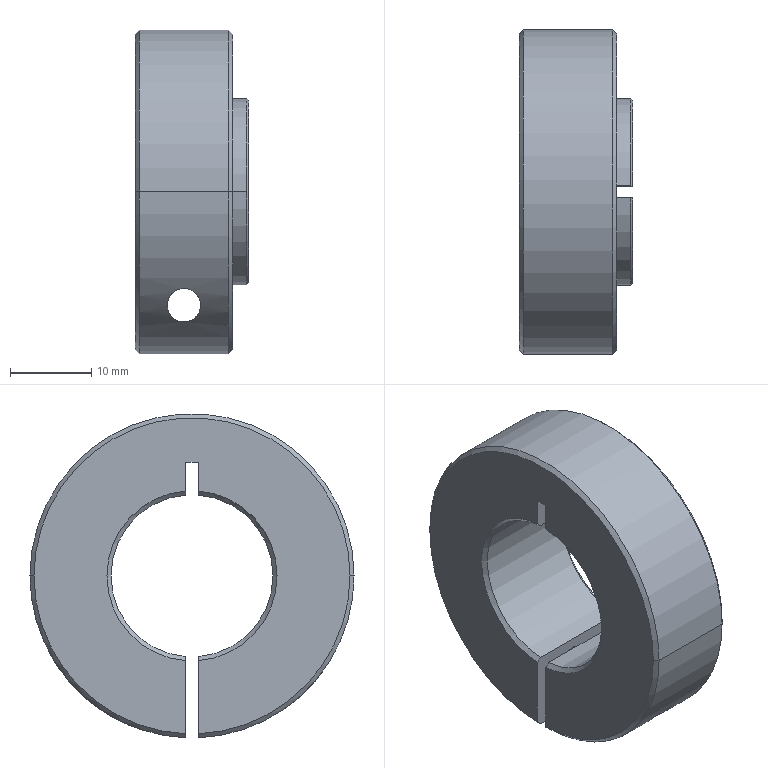Part | NX | features 1_11 2 | 1 solid | 42 faces | box 14 x 40 x 39.986 mm | volume 10434 mm3 | cone 17 | cylinder 15 | plane 10 | commonest cylinder face diameters 20 x3 23 x3 40 x3 4.134 x2 5.5 x2 9 x2
STEP:
#1=CARTESIAN_POINT('',(-38.25,-260.05,-709.529));
#2=VERTEX_POINT('',#1);
#3=CARTESIAN_POINT('',(-32.75,-260.05,-709.529));
#4=VERTEX_POINT('',#3);
#5=CARTESIAN_POINT('',(-35.5,-260.05,-709.529));
#6=DIRECTION('',(0.,1.,0.));
#7=DIRECTION('',(-1.,0.,0.));
#8=AXIS2_PLACEMENT_3D('',#5,#6,#7);
#9=CIRCLE('',#8,2.75);
#10=EDGE_CURVE('',#2,#4,#9,.T.);
#11=ORIENTED_EDGE('',*,*,#10,.F.);
#12=CARTESIAN_POINT('',(-38.25,-253.8,-709.529));
#13=VERTEX_POINT('',#12);
#14=CARTESIAN_POINT('',(-38.25,-253.8,-709.529));
#15=DIRECTION('',(0.,-1.,0.));
#16=VECTOR('',#15,1000.);
#17=LINE('',#14,#16);
#18=EDGE_CURVE('',#13,#2,#17,.T.);
#19=ORIENTED_EDGE('',*,*,#18,.F.);
#20=CARTESIAN_POINT('',(-32.75,-253.8,-709.529));
#21=VERTEX_POINT('',#20);
#22=CARTESIAN_POINT('',(-35.5,-253.8,-709.529));
#23=DIRECTION('',(0.,-1.,0.));
#24=DIRECTION('',(1.,0.,0.));
#25=AXIS2_PLACEMENT_3D('',#22,#23,#24);
#26=CIRCLE('',#25,2.75);
#27=EDGE_CURVE('',#21,#13,#26,.T.);
#28=ORIENTED_EDGE('',*,*,#27,.F.);
#29=CARTESIAN_POINT('',(-32.75,-253.8,-709.529));
#30=DIRECTION('',(0.,-1.,0.));
#31=VECTOR('',#30,1000.);
#32=LINE('',#29,#31);
#33=EDGE_CURVE('',#4,#21,#32,.F.);
#34=ORIENTED_EDGE('',*,*,#33,.F.);
#35=EDGE_LOOP('',(#11,#19,#28,#34));
#36=FACE_BOUND('',#35,.T.);
#37=CARTESIAN_POINT('',(-35.5,-257.3,-709.529));
#38=DIRECTION('',(0.,1.,0.));
#39=DIRECTION('',(-1.,0.,0.));
#40=AXIS2_PLACEMENT_3D('',#37,#38,#39);
#41=CYLINDRICAL_SURFACE('',#40,2.75);
#42=ADVANCED_FACE('',(#36),#41,.F.);
#43=CARTESIAN_POINT('',(-27.5,-261.55,-684.279));
#44=VERTEX_POINT('',#43);
#45=CARTESIAN_POINT('',(-27.5,-272.075,-695.529));
#46=VERTEX_POINT('',#45);
#47=CARTESIAN_POINT('',(-27.5,-260.8,-695.529));
#48=DIRECTION('',(1.,0.,0.));
#49=DIRECTION('',(0.,-0.06652,0.9978));
#50=AXIS2_PLACEMENT_3D('',#47,#48,#49);
#51=CIRCLE('',#50,11.275);
#52=EDGE_CURVE('',#44,#46,#51,.T.);
#53=ORIENTED_EDGE('',*,*,#52,.F.);
#54=CARTESIAN_POINT('',(-27.725,-261.55,-684.054));
#55=VERTEX_POINT('',#54);
#56=CARTESIAN_POINT('',(-27.725,-261.55,-684.054));
#57=CARTESIAN_POINT('',(-27.65,-261.55,-684.129));
#58=CARTESIAN_POINT('',(-27.575,-261.55,-684.204));
#59=CARTESIAN_POINT('',(-27.5,-261.55,-684.279));
#60=B_SPLINE_CURVE_WITH_KNOTS('',3,(#56,#57,#58,#59),.UNSPECIFIED.,.F.,.F.,(4,4),(0.,1.),.UNSPECIFIED.);
#61=EDGE_CURVE('',#44,#55,#60,.F.);
#62=ORIENTED_EDGE('',*,*,#61,.T.);
#63=CARTESIAN_POINT('',(-27.725,-272.3,-695.529));
#64=VERTEX_POINT('',#63);
#65=CARTESIAN_POINT('',(-27.725,-260.8,-695.529));
#66=DIRECTION('',(1.,0.,0.));
#67=DIRECTION('',(0.,-0.06522,0.9979));
#68=AXIS2_PLACEMENT_3D('',#65,#66,#67);
#69=CIRCLE('',#68,11.5);
#70=EDGE_CURVE('',#55,#64,#69,.T.);
#71=ORIENTED_EDGE('',*,*,#70,.T.);
#72=CARTESIAN_POINT('',(-27.725,-272.3,-695.529));
#73=DIRECTION('',(0.7071,0.7071,0.));
#74=VECTOR('',#73,1000.);
#75=LINE('',#72,#74);
#76=EDGE_CURVE('',#64,#46,#75,.T.);
#77=ORIENTED_EDGE('',*,*,#76,.T.);
#78=EDGE_LOOP('',(#53,#62,#71,#77));
#79=FACE_BOUND('',#78,.T.);
#80=CARTESIAN_POINT('',(-27.451,-260.8,-695.529));
#81=DIRECTION('',(-1.,0.,0.));
#82=DIRECTION('',(0.,-1.,0.));
#83=AXIS2_PLACEMENT_3D('',#80,#81,#82);
#84=CONICAL_SURFACE('',#83,11.226,0.7854);
#85=ADVANCED_FACE('',(#79),#84,.T.);
#86=CARTESIAN_POINT('',(-29.5,-260.05,-715.015));
#87=VERTEX_POINT('',#86);
#88=CARTESIAN_POINT('',(-29.5,-241.3,-695.529));
#89=VERTEX_POINT('',#88);
#90=CARTESIAN_POINT('',(-29.5,-260.8,-695.529));
#91=DIRECTION('',(1.,0.,0.));
#92=DIRECTION('',(0.,0.03846,-0.9993));
#93=AXIS2_PLACEMENT_3D('',#90,#91,#92);
#94=CIRCLE('',#93,19.5);
#95=EDGE_CURVE('',#87,#89,#94,.T.);
#96=ORIENTED_EDGE('',*,*,#95,.F.);
#97=CARTESIAN_POINT('',(-30.,-260.05,-715.515));
#98=VERTEX_POINT('',#97);
#99=CARTESIAN_POINT('',(-30.,-260.05,-715.515));
#100=CARTESIAN_POINT('',(-29.833,-260.05,-715.349));
#101=CARTESIAN_POINT('',(-29.667,-260.05,-715.182));
#102=CARTESIAN_POINT('',(-29.5,-260.05,-715.015));
#103=B_SPLINE_CURVE_WITH_KNOTS('',3,(#99,#100,#101,#102),.UNSPECIFIED.,.F.,.F.,(4,4),(0.,1.),.UNSPECIFIED.);
#104=EDGE_CURVE('',#87,#98,#103,.F.);
#105=ORIENTED_EDGE('',*,*,#104,.T.);
#106=CARTESIAN_POINT('',(-30.,-240.8,-695.529));
#107=VERTEX_POINT('',#106);
#108=CARTESIAN_POINT('',(-30.,-260.8,-695.529));
#109=DIRECTION('',(1.,0.,0.));
#110=DIRECTION('',(0.,0.0375,-0.9993));
#111=AXIS2_PLACEMENT_3D('',#108,#109,#110);
#112=CIRCLE('',#111,20.);
#113=EDGE_CURVE('',#98,#107,#112,.T.);
#114=ORIENTED_EDGE('',*,*,#113,.T.);
#115=CARTESIAN_POINT('',(-30.,-240.8,-695.529));
#116=DIRECTION('',(0.7071,-0.7071,0.));
#117=VECTOR('',#116,1000.);
#118=LINE('',#115,#117);
#119=EDGE_CURVE('',#107,#89,#118,.T.);
#120=ORIENTED_EDGE('',*,*,#119,.T.);
#121=EDGE_LOOP('',(#96,#105,#114,#120));
#122=FACE_BOUND('',#121,.T.);
#123=CARTESIAN_POINT('',(-29.451,-260.8,-695.529));
#124=DIRECTION('',(-1.,0.,0.));
#125=DIRECTION('',(0.,-1.,0.));
#126=AXIS2_PLACEMENT_3D('',#123,#124,#125);
#127=CONICAL_SURFACE('',#126,19.451,0.7854);
#128=ADVANCED_FACE('',(#122),#127,.T.);
#129=CARTESIAN_POINT('',(-33.433,-261.983,-709.529));
#130=VERTEX_POINT('',#129);
#131=CARTESIAN_POINT('',(-37.567,-261.983,-709.529));
#132=VERTEX_POINT('',#131);
#133=CARTESIAN_POINT('',(-35.5,-261.983,-709.529));
#134=DIRECTION('',(0.,-1.,0.));
#135=DIRECTION('',(1.,0.,0.));
#136=AXIS2_PLACEMENT_3D('',#133,#134,#135);
#137=CIRCLE('',#136,2.067);
#138=EDGE_CURVE('',#130,#132,#137,.T.);
#139=ORIENTED_EDGE('',*,*,#138,.F.);
#140=CARTESIAN_POINT('',(-33.433,-275.083,-709.529));
#141=VERTEX_POINT('',#140);
#142=CARTESIAN_POINT('',(-33.433,-275.083,-709.529));
#143=DIRECTION('',(0.,1.,0.));
#144=VECTOR('',#143,1000.);
#145=LINE('',#142,#144);
#146=EDGE_CURVE('',#141,#130,#145,.T.);
#147=ORIENTED_EDGE('',*,*,#146,.F.);
#148=CARTESIAN_POINT('',(-37.567,-275.083,-709.529));
#149=VERTEX_POINT('',#148);
#150=CARTESIAN_POINT('',(-37.567,-275.083,-709.529));
#151=CARTESIAN_POINT('',(-37.567,-275.524,-709.078));
#152=CARTESIAN_POINT('',(-37.348,-276.166,-708.351));
#153=CARTESIAN_POINT('',(-36.445,-276.738,-707.615));
#154=CARTESIAN_POINT('',(-35.5,-276.906,-707.386));
#155=CARTESIAN_POINT('',(-34.555,-276.738,-707.615));
#156=CARTESIAN_POINT('',(-33.652,-276.166,-708.351));
#157=CARTESIAN_POINT('',(-33.433,-275.524,-709.078));
#158=CARTESIAN_POINT('',(-33.433,-275.083,-709.529));
#159=B_SPLINE_CURVE_WITH_KNOTS('',3,(#150,#151,#152,#153,#154,#155,#156,#157,#158),.UNSPECIFIED.,.F.,.F.,(4,1,1,1,1,1,4),(0.,0.25,0.375,0.5,0.625,0.75,1.),.UNSPECIFIED.);
#160=EDGE_CURVE('',#141,#149,#159,.F.);
#161=ORIENTED_EDGE('',*,*,#160,.T.);
#162=CARTESIAN_POINT('',(-37.567,-275.083,-709.529));
#163=DIRECTION('',(0.,1.,0.));
#164=VECTOR('',#163,1000.);
#165=LINE('',#162,#164);
#166=EDGE_CURVE('',#132,#149,#165,.F.);
#167=ORIENTED_EDGE('',*,*,#166,.F.);
#168=EDGE_LOOP('',(#139,#147,#161,#167));
#169=FACE_BOUND('',#168,.T.);
#170=CARTESIAN_POINT('',(-35.5,-272.267,-709.529));
#171=DIRECTION('',(0.,-1.,0.));
#172=DIRECTION('',(1.,0.,0.));
#173=AXIS2_PLACEMENT_3D('',#170,#171,#172);
#174=CYLINDRICAL_SURFACE('',#173,2.067);
#175=ADVANCED_FACE('',(#169),#174,.F.);
#176=ORIENTED_EDGE('',*,*,#138,.T.);
#177=CARTESIAN_POINT('',(-38.,-261.55,-709.529));
#178=VERTEX_POINT('',#177);
#179=CARTESIAN_POINT('',(-38.,-261.55,-709.529));
#180=DIRECTION('',(0.7071,-0.7071,0.));
#181=VECTOR('',#180,1000.);
#182=LINE('',#179,#181);
#183=EDGE_CURVE('',#178,#132,#182,.T.);
#184=ORIENTED_EDGE('',*,*,#183,.F.);
#185=CARTESIAN_POINT('',(-33.,-261.55,-709.529));
#186=VERTEX_POINT('',#185);
#187=CARTESIAN_POINT('',(-35.5,-261.55,-709.529));
#188=DIRECTION('',(0.,-1.,0.));
#189=DIRECTION('',(1.,0.,0.));
#190=AXIS2_PLACEMENT_3D('',#187,#188,#189);
#191=CIRCLE('',#190,2.5);
#192=EDGE_CURVE('',#186,#178,#191,.T.);
#193=ORIENTED_EDGE('',*,*,#192,.F.);
#194=CARTESIAN_POINT('',(-33.,-261.55,-709.529));
#195=DIRECTION('',(-0.7071,-0.7071,0.));
#196=VECTOR('',#195,1000.);
#197=LINE('',#194,#196);
#198=EDGE_CURVE('',#130,#186,#197,.F.);
#199=ORIENTED_EDGE('',*,*,#198,.F.);
#200=EDGE_LOOP('',(#176,#184,#193,#199));
#201=FACE_BOUND('',#200,.T.);
#202=CARTESIAN_POINT('',(-35.5,-262.032,-709.529));
#203=DIRECTION('',(0.,1.,0.));
#204=DIRECTION('',(-1.,0.,0.));
#205=AXIS2_PLACEMENT_3D('',#202,#203,#204);
#206=CONICAL_SURFACE('',#205,2.018,0.7854);
#207=ADVANCED_FACE('',(#201),#206,.F.);
#208=ORIENTED_EDGE('',*,*,#198,.T.);
#209=CARTESIAN_POINT('',(-35.5,-261.55,-709.529));
#210=DIRECTION('',(0.,-1.,0.));
#211=DIRECTION('',(-1.,0.,0.));
#212=AXIS2_PLACEMENT_3D('',#209,#210,#211);
#213=CIRCLE('',#212,2.5);
#214=EDGE_CURVE('',#178,#186,#213,.T.);
#215=ORIENTED_EDGE('',*,*,#214,.F.);
#216=ORIENTED_EDGE('',*,*,#183,.T.);
#217=CARTESIAN_POINT('',(-35.5,-261.983,-709.529));
#218=DIRECTION('',(0.,-1.,0.));
#219=DIRECTION('',(-1.,0.,0.));
#220=AXIS2_PLACEMENT_3D('',#217,#218,#219);
#221=CIRCLE('',#220,2.067);
#222=EDGE_CURVE('',#132,#130,#221,.T.);
#223=ORIENTED_EDGE('',*,*,#222,.T.);
#224=EDGE_LOOP('',(#208,#215,#216,#223));
#225=FACE_BOUND('',#224,.T.);
#226=CARTESIAN_POINT('',(-35.5,-262.032,-709.529));
#227=DIRECTION('',(0.,1.,0.));
#228=DIRECTION('',(-1.,0.,0.));
#229=AXIS2_PLACEMENT_3D('',#226,#227,#228);
#230=CONICAL_SURFACE('',#229,2.018,0.7854);
#231=ADVANCED_FACE('',(#225),#230,.F.);
#232=ORIENTED_EDGE('',*,*,#166,.T.);
#233=CARTESIAN_POINT('',(-33.433,-275.083,-709.529));
#234=CARTESIAN_POINT('',(-33.433,-274.603,-710.02));
#235=CARTESIAN_POINT('',(-33.683,-273.842,-710.714));
#236=CARTESIAN_POINT('',(-34.497,-272.96,-711.413));
#237=CARTESIAN_POINT('',(-35.5,-272.586,-711.688));
#238=CARTESIAN_POINT('',(-36.503,-272.96,-711.413));
#239=CARTESIAN_POINT('',(-37.317,-273.842,-710.714));
#240=CARTESIAN_POINT('',(-37.567,-274.603,-710.02));
#241=CARTESIAN_POINT('',(-37.567,-275.083,-709.529));
#242=B_SPLINE_CURVE_WITH_KNOTS('',3,(#233,#234,#235,#236,#237,#238,#239,#240,#241),.UNSPECIFIED.,.F.,.F.,(4,1,1,1,1,1,4),(0.,0.25,0.375,0.5,0.625,0.75,1.),.UNSPECIFIED.);
#243=EDGE_CURVE('',#149,#141,#242,.F.);
#244=ORIENTED_EDGE('',*,*,#243,.T.);
#245=ORIENTED_EDGE('',*,*,#146,.T.);
#246=ORIENTED_EDGE('',*,*,#222,.F.);
#247=EDGE_LOOP('',(#232,#244,#245,#246));
#248=FACE_BOUND('',#247,.T.);
#249=CARTESIAN_POINT('',(-35.5,-272.267,-709.529));
#250=DIRECTION('',(0.,-1.,0.));
#251=DIRECTION('',(1.,0.,0.));
#252=AXIS2_PLACEMENT_3D('',#249,#250,#251);
#253=CYLINDRICAL_SURFACE('',#252,2.067);
#254=ADVANCED_FACE('',(#248),#253,.F.);
#255=ORIENTED_EDGE('',*,*,#160,.F.);
#256=ORIENTED_EDGE('',*,*,#243,.F.);
#257=EDGE_LOOP('',(#255,#256));
#258=FACE_BOUND('',#257,.T.);
#259=CARTESIAN_POINT('',(-41.,-280.8,-695.529));
#260=VERTEX_POINT('',#259);
#261=CARTESIAN_POINT('',(-30.,-280.8,-695.529));
#262=VERTEX_POINT('',#261);
#263=CARTESIAN_POINT('',(-41.,-280.8,-695.529));
#264=DIRECTION('',(1.,0.,0.));
#265=VECTOR('',#264,1000.);
#266=LINE('',#263,#265);
#267=EDGE_CURVE('',#260,#262,#266,.T.);
#268=ORIENTED_EDGE('',*,*,#267,.F.);
#269=CARTESIAN_POINT('',(-41.,-261.55,-715.515));
#270=VERTEX_POINT('',#269);
#271=CARTESIAN_POINT('',(-41.,-260.8,-695.529));
#272=DIRECTION('',(-1.,0.,0.));
#273=DIRECTION('',(0.,-0.0375,-0.9993));
#274=AXIS2_PLACEMENT_3D('',#271,#272,#273);
#275=CIRCLE('',#274,20.);
#276=EDGE_CURVE('',#270,#260,#275,.T.);
#277=ORIENTED_EDGE('',*,*,#276,.F.);
#278=CARTESIAN_POINT('',(-30.,-261.55,-715.515));
#279=VERTEX_POINT('',#278);
#280=CARTESIAN_POINT('',(-41.,-261.55,-715.515));
#281=DIRECTION('',(1.,0.,0.));
#282=VECTOR('',#281,1000.);
#283=LINE('',#280,#282);
#284=EDGE_CURVE('',#270,#279,#283,.T.);
#285=ORIENTED_EDGE('',*,*,#284,.T.);
#286=CARTESIAN_POINT('',(-30.,-260.8,-695.529));
#287=DIRECTION('',(1.,0.,0.));
#288=DIRECTION('',(0.,-1.,0.));
#289=AXIS2_PLACEMENT_3D('',#286,#287,#288);
#290=CIRCLE('',#289,20.);
#291=EDGE_CURVE('',#262,#279,#290,.T.);
#292=ORIENTED_EDGE('',*,*,#291,.F.);
#293=EDGE_LOOP('',(#268,#277,#285,#292));
#294=FACE_BOUND('',#293,.T.);
#295=CARTESIAN_POINT('',(-35.5,-260.8,-695.529));
#296=DIRECTION('',(-1.,0.,0.));
#297=DIRECTION('',(0.,-1.,0.));
#298=AXIS2_PLACEMENT_3D('',#295,#296,#297);
#299=CYLINDRICAL_SURFACE('',#298,20.);
#300=ADVANCED_FACE('',(#258,#294),#299,.T.);
#301=CARTESIAN_POINT('',(-29.5,-280.3,-695.529));
#302=VERTEX_POINT('',#301);
#303=CARTESIAN_POINT('',(-30.,-280.8,-695.529));
#304=DIRECTION('',(0.7071,0.7071,0.));
#305=VECTOR('',#304,1000.);
#306=LINE('',#303,#305);
#307=EDGE_CURVE('',#262,#302,#306,.T.);
#308=ORIENTED_EDGE('',*,*,#307,.F.);
#309=ORIENTED_EDGE('',*,*,#291,.T.);
#310=CARTESIAN_POINT('',(-29.5,-261.55,-715.015));
#311=VERTEX_POINT('',#310);
#312=CARTESIAN_POINT('',(-29.5,-261.55,-715.015));
#313=CARTESIAN_POINT('',(-29.667,-261.55,-715.182));
#314=CARTESIAN_POINT('',(-29.833,-261.55,-715.349));
#315=CARTESIAN_POINT('',(-30.,-261.55,-715.515));
#316=B_SPLINE_CURVE_WITH_KNOTS('',3,(#312,#313,#314,#315),.UNSPECIFIED.,.F.,.F.,(4,4),(0.,1.),.UNSPECIFIED.);
#317=EDGE_CURVE('',#279,#311,#316,.F.);
#318=ORIENTED_EDGE('',*,*,#317,.T.);
#319=CARTESIAN_POINT('',(-29.5,-260.8,-695.529));
#320=DIRECTION('',(1.,0.,0.));
#321=DIRECTION('',(0.,-1.,0.));
#322=AXIS2_PLACEMENT_3D('',#319,#320,#321);
#323=CIRCLE('',#322,19.5);
#324=EDGE_CURVE('',#302,#311,#323,.T.);
#325=ORIENTED_EDGE('',*,*,#324,.F.);
#326=EDGE_LOOP('',(#308,#309,#318,#325));
#327=FACE_BOUND('',#326,.T.);
#328=CARTESIAN_POINT('',(-29.451,-260.8,-695.529));
#329=DIRECTION('',(-1.,0.,0.));
#330=DIRECTION('',(0.,-1.,0.));
#331=AXIS2_PLACEMENT_3D('',#328,#329,#330);
#332=CONICAL_SURFACE('',#331,19.451,0.7854);
#333=ADVANCED_FACE('',(#327),#332,.T.);
#334=CARTESIAN_POINT('',(-41.5,-261.55,-681.529));
#335=VERTEX_POINT('',#334);
#336=CARTESIAN_POINT('',(-41.5,-260.05,-681.529));
#337=VERTEX_POINT('',#336);
#338=CARTESIAN_POINT('',(-41.5,-261.55,-681.529));
#339=DIRECTION('',(0.,1.,0.));
#340=VECTOR('',#339,1000.);
#341=LINE('',#338,#340);
#342=EDGE_CURVE('',#335,#337,#341,.T.);
#343=ORIENTED_EDGE('',*,*,#342,.T.);
#344=CARTESIAN_POINT('',(-29.5,-260.05,-681.529));
#345=VERTEX_POINT('',#344);
#346=CARTESIAN_POINT('',(-29.5,-260.05,-681.529));
#347=DIRECTION('',(-1.,0.,0.));
#348=VECTOR('',#347,1000.);
#349=LINE('',#346,#348);
#350=EDGE_CURVE('',#345,#337,#349,.T.);
#351=ORIENTED_EDGE('',*,*,#350,.F.);
#352=CARTESIAN_POINT('',(-29.5,-261.55,-681.529));
#353=VERTEX_POINT('',#352);
#354=CARTESIAN_POINT('',(-29.5,-260.05,-681.529));
#355=DIRECTION('',(0.,-1.,0.));
#356=VECTOR('',#355,1000.);
#357=LINE('',#354,#356);
#358=EDGE_CURVE('',#345,#353,#357,.T.);
#359=ORIENTED_EDGE('',*,*,#358,.T.);
#360=CARTESIAN_POINT('',(-41.5,-261.55,-681.529));
#361=DIRECTION('',(1.,0.,0.));
#362=VECTOR('',#361,1000.);
#363=LINE('',#360,#362);
#364=EDGE_CURVE('',#335,#353,#363,.T.);
#365=ORIENTED_EDGE('',*,*,#364,.F.);
#366=EDGE_LOOP('',(#343,#351,#359,#365));
#367=FACE_BOUND('',#366,.T.);
#368=CARTESIAN_POINT('',(-59.5,-261.55,-681.529));
#369=DIRECTION('',(0.,0.,1.));
#370=DIRECTION('',(0.,1.,0.));
#371=AXIS2_PLACEMENT_3D('',#368,#369,#370);
#372=PLANE('',#371);
#373=ADVANCED_FACE('',(#367),#372,.F.);
#374=CARTESIAN_POINT('',(-41.5,-260.05,-685.056));
#375=VERTEX_POINT('',#374);
#376=CARTESIAN_POINT('',(-41.5,-260.05,-681.529));
#377=DIRECTION('',(0.,0.,-1.));
#378=VECTOR('',#377,1000.);
#379=LINE('',#376,#378);
#380=EDGE_CURVE('',#337,#375,#379,.T.);
#381=ORIENTED_EDGE('',*,*,#380,.T.);
#382=CARTESIAN_POINT('',(-41.,-260.05,-685.558));
#383=VERTEX_POINT('',#382);
#384=CARTESIAN_POINT('',(-41.5,-260.05,-685.056));
#385=CARTESIAN_POINT('',(-41.333,-260.05,-685.223));
#386=CARTESIAN_POINT('',(-41.167,-260.05,-685.39));
#387=CARTESIAN_POINT('',(-41.,-260.05,-685.558));
#388=B_SPLINE_CURVE_WITH_KNOTS('',3,(#384,#385,#386,#387),.UNSPECIFIED.,.F.,.F.,(4,4),(0.,1.),.UNSPECIFIED.);
#389=EDGE_CURVE('',#383,#375,#388,.F.);
#390=ORIENTED_EDGE('',*,*,#389,.F.);
#391=CARTESIAN_POINT('',(-28.,-260.05,-685.558));
#392=VERTEX_POINT('',#391);
#393=CARTESIAN_POINT('',(-28.,-260.05,-685.558));
#394=DIRECTION('',(-1.,0.,0.));
#395=VECTOR('',#394,1000.);
#396=LINE('',#393,#395);
#397=EDGE_CURVE('',#392,#383,#396,.T.);
#398=ORIENTED_EDGE('',*,*,#397,.F.);
#399=CARTESIAN_POINT('',(-27.5,-260.05,-685.056));
#400=VERTEX_POINT('',#399);
#401=CARTESIAN_POINT('',(-28.,-260.05,-685.558));
#402=CARTESIAN_POINT('',(-27.833,-260.05,-685.39));
#403=CARTESIAN_POINT('',(-27.667,-260.05,-685.223));
#404=CARTESIAN_POINT('',(-27.5,-260.05,-685.056));
#405=B_SPLINE_CURVE_WITH_KNOTS('',3,(#401,#402,#403,#404),.UNSPECIFIED.,.F.,.F.,(4,4),(0.,1.),.UNSPECIFIED.);
#406=EDGE_CURVE('',#400,#392,#405,.F.);
#407=ORIENTED_EDGE('',*,*,#406,.F.);
#408=CARTESIAN_POINT('',(-27.5,-260.05,-684.279));
#409=VERTEX_POINT('',#408);
#410=CARTESIAN_POINT('',(-27.5,-260.05,-685.056));
#411=DIRECTION('',(0.,0.,1.));
#412=VECTOR('',#411,1000.);
#413=LINE('',#410,#412);
#414=EDGE_CURVE('',#400,#409,#413,.T.);
#415=ORIENTED_EDGE('',*,*,#414,.T.);
#416=CARTESIAN_POINT('',(-27.725,-260.05,-684.054));
#417=VERTEX_POINT('',#416);
#418=CARTESIAN_POINT('',(-27.5,-260.05,-684.279));
#419=CARTESIAN_POINT('',(-27.575,-260.05,-684.204));
#420=CARTESIAN_POINT('',(-27.65,-260.05,-684.129));
#421=CARTESIAN_POINT('',(-27.725,-260.05,-684.054));
#422=B_SPLINE_CURVE_WITH_KNOTS('',3,(#418,#419,#420,#421),.UNSPECIFIED.,.F.,.F.,(4,4),(0.,1.),.UNSPECIFIED.);
#423=EDGE_CURVE('',#417,#409,#422,.F.);
#424=ORIENTED_EDGE('',*,*,#423,.F.);
#425=CARTESIAN_POINT('',(-29.5,-260.05,-684.054));
#426=VERTEX_POINT('',#425);
#427=CARTESIAN_POINT('',(-29.5,-260.05,-684.054));
#428=DIRECTION('',(1.,0.,0.));
#429=VECTOR('',#428,1000.);
#430=LINE('',#427,#429);
#431=EDGE_CURVE('',#426,#417,#430,.T.);
#432=ORIENTED_EDGE('',*,*,#431,.F.);
#433=CARTESIAN_POINT('',(-29.5,-260.05,-684.054));
#434=DIRECTION('',(0.,0.,1.));
#435=VECTOR('',#434,1000.);
#436=LINE('',#433,#435);
#437=EDGE_CURVE('',#426,#345,#436,.T.);
#438=ORIENTED_EDGE('',*,*,#437,.T.);
#439=ORIENTED_EDGE('',*,*,#350,.T.);
#440=EDGE_LOOP('',(#381,#390,#398,#407,#415,#424,#432,#438,#439));
#441=FACE_BOUND('',#440,.T.);
#442=CARTESIAN_POINT('',(-59.5,-260.05,-681.529));
#443=DIRECTION('',(0.,1.,0.));
#444=DIRECTION('',(-1.,0.,0.));
#445=AXIS2_PLACEMENT_3D('',#442,#443,#444);
#446=PLANE('',#445);
#447=ADVANCED_FACE('',(#441),#446,.F.);
#448=CARTESIAN_POINT('',(-41.,-260.05,-705.501));
#449=VERTEX_POINT('',#448);
#450=CARTESIAN_POINT('',(-41.,-250.8,-695.529));
#451=VERTEX_POINT('',#450);
#452=CARTESIAN_POINT('',(-41.,-260.8,-695.529));
#453=DIRECTION('',(1.,0.,0.));
#454=DIRECTION('',(0.,0.075,-0.9972));
#455=AXIS2_PLACEMENT_3D('',#452,#453,#454);
#456=CIRCLE('',#455,10.);
#457=EDGE_CURVE('',#449,#451,#456,.T.);
#458=ORIENTED_EDGE('',*,*,#457,.F.);
#459=CARTESIAN_POINT('',(-28.,-260.05,-705.501));
#460=VERTEX_POINT('',#459);
#461=CARTESIAN_POINT('',(-41.,-260.05,-705.501));
#462=DIRECTION('',(1.,0.,0.));
#463=VECTOR('',#462,1000.);
#464=LINE('',#461,#463);
#465=EDGE_CURVE('',#449,#460,#464,.T.);
#466=ORIENTED_EDGE('',*,*,#465,.T.);
#467=CARTESIAN_POINT('',(-28.,-250.8,-695.529));
#468=VERTEX_POINT('',#467);
#469=CARTESIAN_POINT('',(-28.,-260.8,-695.529));
#470=DIRECTION('',(-1.,0.,0.));
#471=DIRECTION('',(0.,1.,0.));
#472=AXIS2_PLACEMENT_3D('',#469,#470,#471);
#473=CIRCLE('',#472,10.);
#474=EDGE_CURVE('',#468,#460,#473,.T.);
#475=ORIENTED_EDGE('',*,*,#474,.F.);
#476=CARTESIAN_POINT('',(-28.,-260.8,-695.529));
#477=DIRECTION('',(-1.,0.,0.));
#478=DIRECTION('',(0.,0.075,0.9972));
#479=AXIS2_PLACEMENT_3D('',#476,#477,#478);
#480=CIRCLE('',#479,10.);
#481=EDGE_CURVE('',#392,#468,#480,.T.);
#482=ORIENTED_EDGE('',*,*,#481,.F.);
#483=ORIENTED_EDGE('',*,*,#397,.T.);
#484=CARTESIAN_POINT('',(-41.,-260.8,-695.529));
#485=DIRECTION('',(1.,0.,0.));
#486=DIRECTION('',(0.,1.,0.));
#487=AXIS2_PLACEMENT_3D('',#484,#485,#486);
#488=CIRCLE('',#487,10.);
#489=EDGE_CURVE('',#451,#383,#488,.T.);
#490=ORIENTED_EDGE('',*,*,#489,.F.);
#491=EDGE_LOOP('',(#458,#466,#475,#482,#483,#490));
#492=FACE_BOUND('',#491,.T.);
#493=CARTESIAN_POINT('',(-34.5,-260.8,-695.529));
#494=DIRECTION('',(-1.,0.,0.));
#495=DIRECTION('',(0.,-1.,0.));
#496=AXIS2_PLACEMENT_3D('',#493,#494,#495);
#497=CYLINDRICAL_SURFACE('',#496,10.);
#498=ADVANCED_FACE('',(#492),#497,.F.);
#499=CARTESIAN_POINT('',(-27.5,-250.3,-695.529));
#500=VERTEX_POINT('',#499);
#501=CARTESIAN_POINT('',(-27.5,-250.3,-695.529));
#502=DIRECTION('',(-0.7071,-0.7071,0.));
#503=VECTOR('',#502,1000.);
#504=LINE('',#501,#503);
#505=EDGE_CURVE('',#500,#468,#504,.T.);
#506=ORIENTED_EDGE('',*,*,#505,.F.);
#507=CARTESIAN_POINT('',(-27.5,-260.8,-695.529));
#508=DIRECTION('',(-1.,0.,0.));
#509=DIRECTION('',(0.,0.07143,0.9974));
#510=AXIS2_PLACEMENT_3D('',#507,#508,#509);
#511=CIRCLE('',#510,10.5);
#512=EDGE_CURVE('',#400,#500,#511,.T.);
#513=ORIENTED_EDGE('',*,*,#512,.F.);
#514=ORIENTED_EDGE('',*,*,#406,.T.);
#515=ORIENTED_EDGE('',*,*,#481,.T.);
#516=EDGE_LOOP('',(#506,#513,#514,#515));
#517=FACE_BOUND('',#516,.T.);
#518=CARTESIAN_POINT('',(-28.049,-260.8,-695.529));
#519=DIRECTION('',(1.,0.,0.));
#520=DIRECTION('',(0.,1.,0.));
#521=AXIS2_PLACEMENT_3D('',#518,#519,#520);
#522=CONICAL_SURFACE('',#521,9.951,0.7854);
#523=ADVANCED_FACE('',(#517),#522,.F.);
#524=ORIENTED_EDGE('',*,*,#474,.T.);
#525=CARTESIAN_POINT('',(-27.5,-260.05,-706.003));
#526=VERTEX_POINT('',#525);
#527=CARTESIAN_POINT('',(-27.5,-260.05,-706.003));
#528=CARTESIAN_POINT('',(-27.667,-260.05,-705.835));
#529=CARTESIAN_POINT('',(-27.833,-260.05,-705.668));
#530=CARTESIAN_POINT('',(-28.,-260.05,-705.501));
#531=B_SPLINE_CURVE_WITH_KNOTS('',3,(#527,#528,#529,#530),.UNSPECIFIED.,.F.,.F.,(4,4),(0.,1.),.UNSPECIFIED.);
#532=EDGE_CURVE('',#460,#526,#531,.F.);
#533=ORIENTED_EDGE('',*,*,#532,.T.);
#534=CARTESIAN_POINT('',(-27.5,-260.8,-695.529));
#535=DIRECTION('',(-1.,0.,0.));
#536=DIRECTION('',(0.,1.,0.));
#537=AXIS2_PLACEMENT_3D('',#534,#535,#536);
#538=CIRCLE('',#537,10.5);
#539=EDGE_CURVE('',#500,#526,#538,.T.);
#540=ORIENTED_EDGE('',*,*,#539,.F.);
#541=ORIENTED_EDGE('',*,*,#505,.T.);
#542=EDGE_LOOP('',(#524,#533,#540,#541));
#543=FACE_BOUND('',#542,.T.);
#544=CARTESIAN_POINT('',(-28.049,-260.8,-695.529));
#545=DIRECTION('',(1.,0.,0.));
#546=DIRECTION('',(0.,1.,0.));
#547=AXIS2_PLACEMENT_3D('',#544,#545,#546);
#548=CONICAL_SURFACE('',#547,9.951,0.7854);
#549=ADVANCED_FACE('',(#543),#548,.F.);
#550=CARTESIAN_POINT('',(-27.5,-260.05,-706.779));
#551=VERTEX_POINT('',#550);
#552=CARTESIAN_POINT('',(-27.5,-249.525,-695.529));
#553=VERTEX_POINT('',#552);
#554=CARTESIAN_POINT('',(-27.5,-260.8,-695.529));
#555=DIRECTION('',(1.,0.,0.));
#556=DIRECTION('',(0.,0.06652,-0.9978));
#557=AXIS2_PLACEMENT_3D('',#554,#555,#556);
#558=CIRCLE('',#557,11.275);
#559=EDGE_CURVE('',#551,#553,#558,.T.);
#560=ORIENTED_EDGE('',*,*,#559,.T.);
#561=CARTESIAN_POINT('',(-27.5,-260.8,-695.529));
#562=DIRECTION('',(1.,0.,0.));
#563=DIRECTION('',(0.,1.,0.));
#564=AXIS2_PLACEMENT_3D('',#561,#562,#563);
#565=CIRCLE('',#564,11.275);
#566=EDGE_CURVE('',#553,#409,#565,.T.);
#567=ORIENTED_EDGE('',*,*,#566,.T.);
#568=ORIENTED_EDGE('',*,*,#414,.F.);
#569=ORIENTED_EDGE('',*,*,#512,.T.);
#570=ORIENTED_EDGE('',*,*,#539,.T.);
#571=CARTESIAN_POINT('',(-27.5,-260.05,-706.779));
#572=DIRECTION('',(0.,0.,1.));
#573=VECTOR('',#572,1000.);
#574=LINE('',#571,#573);
#575=EDGE_CURVE('',#551,#526,#574,.T.);
#576=ORIENTED_EDGE('',*,*,#575,.F.);
#577=EDGE_LOOP('',(#560,#567,#568,#569,#570,#576));
#578=FACE_BOUND('',#577,.T.);
#579=CARTESIAN_POINT('',(-27.5,-260.8,-684.642));
#580=DIRECTION('',(1.,0.,0.));
#581=DIRECTION('',(0.,1.,0.));
#582=AXIS2_PLACEMENT_3D('',#579,#580,#581);
#583=PLANE('',#582);
#584=ADVANCED_FACE('',(#578),#583,.T.);
#585=CARTESIAN_POINT('',(-27.725,-260.05,-707.005));
#586=VERTEX_POINT('',#585);
#587=CARTESIAN_POINT('',(-27.725,-249.3,-695.529));
#588=VERTEX_POINT('',#587);
#589=CARTESIAN_POINT('',(-27.725,-260.8,-695.529));
#590=DIRECTION('',(1.,0.,0.));
#591=DIRECTION('',(0.,0.06522,-0.9979));
#592=AXIS2_PLACEMENT_3D('',#589,#590,#591);
#593=CIRCLE('',#592,11.5);
#594=EDGE_CURVE('',#586,#588,#593,.T.);
#595=ORIENTED_EDGE('',*,*,#594,.T.);
#596=CARTESIAN_POINT('',(-27.725,-260.8,-695.529));
#597=DIRECTION('',(1.,0.,0.));
#598=DIRECTION('',(0.,1.,0.));
#599=AXIS2_PLACEMENT_3D('',#596,#597,#598);
#600=CIRCLE('',#599,11.5);
#601=EDGE_CURVE('',#588,#417,#600,.T.);
#602=ORIENTED_EDGE('',*,*,#601,.T.);
#603=ORIENTED_EDGE('',*,*,#423,.T.);
#604=ORIENTED_EDGE('',*,*,#566,.F.);
#605=ORIENTED_EDGE('',*,*,#559,.F.);
#606=CARTESIAN_POINT('',(-27.725,-260.05,-707.005));
#607=CARTESIAN_POINT('',(-27.65,-260.05,-706.93));
#608=CARTESIAN_POINT('',(-27.575,-260.05,-706.855));
#609=CARTESIAN_POINT('',(-27.5,-260.05,-706.779));
#610=B_SPLINE_CURVE_WITH_KNOTS('',3,(#606,#607,#608,#609),.UNSPECIFIED.,.F.,.F.,(4,4),(0.,1.),.UNSPECIFIED.);
#611=EDGE_CURVE('',#551,#586,#610,.F.);
#612=ORIENTED_EDGE('',*,*,#611,.T.);
#613=EDGE_LOOP('',(#595,#602,#603,#604,#605,#612));
#614=FACE_BOUND('',#613,.T.);
#615=CARTESIAN_POINT('',(-27.451,-260.8,-695.529));
#616=DIRECTION('',(-1.,0.,0.));
#617=DIRECTION('',(0.,-1.,0.));
#618=AXIS2_PLACEMENT_3D('',#615,#616,#617);
#619=CONICAL_SURFACE('',#618,11.226,0.7854);
#620=ADVANCED_FACE('',(#614),#619,.T.);
#621=CARTESIAN_POINT('',(-29.5,-249.3,-695.529));
#622=VERTEX_POINT('',#621);
#623=CARTESIAN_POINT('',(-29.5,-260.05,-707.005));
#624=VERTEX_POINT('',#623);
#625=CARTESIAN_POINT('',(-29.5,-260.8,-695.529));
#626=DIRECTION('',(-1.,0.,0.));
#627=DIRECTION('',(0.,1.,0.));
#628=AXIS2_PLACEMENT_3D('',#625,#626,#627);
#629=CIRCLE('',#628,11.5);
#630=EDGE_CURVE('',#622,#624,#629,.T.);
#631=ORIENTED_EDGE('',*,*,#630,.F.);
#632=CARTESIAN_POINT('',(-29.5,-260.8,-695.529));
#633=DIRECTION('',(-1.,0.,0.));
#634=DIRECTION('',(0.,0.06522,0.9979));
#635=AXIS2_PLACEMENT_3D('',#632,#633,#634);
#636=CIRCLE('',#635,11.5);
#637=EDGE_CURVE('',#426,#622,#636,.T.);
#638=ORIENTED_EDGE('',*,*,#637,.F.);
#639=ORIENTED_EDGE('',*,*,#431,.T.);
#640=ORIENTED_EDGE('',*,*,#601,.F.);
#641=ORIENTED_EDGE('',*,*,#594,.F.);
#642=CARTESIAN_POINT('',(-27.725,-260.05,-707.005));
#643=DIRECTION('',(-1.,0.,0.));
#644=VECTOR('',#643,1000.);
#645=LINE('',#642,#644);
#646=EDGE_CURVE('',#586,#624,#645,.T.);
#647=ORIENTED_EDGE('',*,*,#646,.T.);
#648=EDGE_LOOP('',(#631,#638,#639,#640,#641,#647));
#649=FACE_BOUND('',#648,.T.);
#650=CARTESIAN_POINT('',(-28.613,-260.8,-695.529));
#651=DIRECTION('',(-1.,0.,0.));
#652=DIRECTION('',(0.,-1.,0.));
#653=AXIS2_PLACEMENT_3D('',#650,#651,#652);
#654=CYLINDRICAL_SURFACE('',#653,11.5);
#655=ADVANCED_FACE('',(#649),#654,.T.);
#656=ORIENTED_EDGE('',*,*,#95,.T.);
#657=CARTESIAN_POINT('',(-29.5,-260.8,-695.529));
#658=DIRECTION('',(1.,0.,0.));
#659=DIRECTION('',(0.,1.,0.));
#660=AXIS2_PLACEMENT_3D('',#657,#658,#659);
#661=CIRCLE('',#660,19.5);
#662=EDGE_CURVE('',#89,#302,#661,.T.);
#663=ORIENTED_EDGE('',*,*,#662,.T.);
#664=ORIENTED_EDGE('',*,*,#324,.T.);
#665=CARTESIAN_POINT('',(-29.5,-261.55,-707.005));
#666=VERTEX_POINT('',#665);
#667=CARTESIAN_POINT('',(-29.5,-261.55,-707.005));
#668=DIRECTION('',(0.,0.,-1.));
#669=VECTOR('',#668,1000.);
#670=LINE('',#667,#669);
#671=EDGE_CURVE('',#666,#311,#670,.T.);
#672=ORIENTED_EDGE('',*,*,#671,.F.);
#673=CARTESIAN_POINT('',(-29.5,-272.3,-695.529));
#674=VERTEX_POINT('',#673);
#675=CARTESIAN_POINT('',(-29.5,-260.8,-695.529));
#676=DIRECTION('',(-1.,0.,0.));
#677=DIRECTION('',(0.,-0.06522,-0.9979));
#678=AXIS2_PLACEMENT_3D('',#675,#676,#677);
#679=CIRCLE('',#678,11.5);
#680=EDGE_CURVE('',#666,#674,#679,.T.);
#681=ORIENTED_EDGE('',*,*,#680,.T.);
#682=CARTESIAN_POINT('',(-29.5,-261.55,-684.054));
#683=VERTEX_POINT('',#682);
#684=CARTESIAN_POINT('',(-29.5,-260.8,-695.529));
#685=DIRECTION('',(-1.,0.,0.));
#686=DIRECTION('',(0.,-1.,0.));
#687=AXIS2_PLACEMENT_3D('',#684,#685,#686);
#688=CIRCLE('',#687,11.5);
#689=EDGE_CURVE('',#674,#683,#688,.T.);
#690=ORIENTED_EDGE('',*,*,#689,.T.);
#691=CARTESIAN_POINT('',(-29.5,-261.55,-681.529));
#692=DIRECTION('',(0.,0.,-1.));
#693=VECTOR('',#692,1000.);
#694=LINE('',#691,#693);
#695=EDGE_CURVE('',#353,#683,#694,.T.);
#696=ORIENTED_EDGE('',*,*,#695,.F.);
#697=ORIENTED_EDGE('',*,*,#358,.F.);
#698=ORIENTED_EDGE('',*,*,#437,.F.);
#699=ORIENTED_EDGE('',*,*,#637,.T.);
#700=ORIENTED_EDGE('',*,*,#630,.T.);
#701=CARTESIAN_POINT('',(-29.5,-260.05,-715.015));
#702=DIRECTION('',(0.,0.,1.));
#703=VECTOR('',#702,1000.);
#704=LINE('',#701,#703);
#705=EDGE_CURVE('',#87,#624,#704,.T.);
#706=ORIENTED_EDGE('',*,*,#705,.F.);
#707=EDGE_LOOP('',(#656,#663,#664,#672,#681,#690,#696,#697,#698,#699,#700,#706));
#708=FACE_BOUND('',#707,.T.);
#709=CARTESIAN_POINT('',(-29.5,-260.8,-680.029));
#710=DIRECTION('',(1.,0.,0.));
#711=DIRECTION('',(0.,1.,0.));
#712=AXIS2_PLACEMENT_3D('',#709,#710,#711);
#713=PLANE('',#712);
#714=ADVANCED_FACE('',(#708),#713,.T.);
#715=ORIENTED_EDGE('',*,*,#119,.F.);
#716=CARTESIAN_POINT('',(-30.,-260.8,-695.529));
#717=DIRECTION('',(1.,0.,0.));
#718=DIRECTION('',(0.,1.,0.));
#719=AXIS2_PLACEMENT_3D('',#716,#717,#718);
#720=CIRCLE('',#719,20.);
#721=EDGE_CURVE('',#107,#262,#720,.T.);
#722=ORIENTED_EDGE('',*,*,#721,.T.);
#723=ORIENTED_EDGE('',*,*,#307,.T.);
#724=ORIENTED_EDGE('',*,*,#662,.F.);
#725=EDGE_LOOP('',(#715,#722,#723,#724));
#726=FACE_BOUND('',#725,.T.);
#727=CARTESIAN_POINT('',(-29.451,-260.8,-695.529));
#728=DIRECTION('',(-1.,0.,0.));
#729=DIRECTION('',(0.,-1.,0.));
#730=AXIS2_PLACEMENT_3D('',#727,#728,#729);
#731=CONICAL_SURFACE('',#730,19.451,0.7854);
#732=ADVANCED_FACE('',(#726),#731,.T.);
#733=CARTESIAN_POINT('',(-41.,-240.8,-695.529));
#734=VERTEX_POINT('',#733);
#735=CARTESIAN_POINT('',(-41.,-240.8,-695.529));
#736=DIRECTION('',(1.,0.,0.));
#737=VECTOR('',#736,1000.);
#738=LINE('',#735,#737);
#739=EDGE_CURVE('',#734,#107,#738,.T.);
#740=ORIENTED_EDGE('',*,*,#739,.F.);
#741=CARTESIAN_POINT('',(-41.,-260.8,-695.529));
#742=DIRECTION('',(-1.,0.,0.));
#743=DIRECTION('',(0.,-1.,0.));
#744=AXIS2_PLACEMENT_3D('',#741,#742,#743);
#745=CIRCLE('',#744,20.);
#746=EDGE_CURVE('',#260,#734,#745,.T.);
#747=ORIENTED_EDGE('',*,*,#746,.F.);
#748=ORIENTED_EDGE('',*,*,#267,.T.);
#749=ORIENTED_EDGE('',*,*,#721,.F.);
#750=EDGE_LOOP('',(#740,#747,#748,#749));
#751=FACE_BOUND('',#750,.T.);
#752=CARTESIAN_POINT('',(-35.5,-260.8,-695.529));
#753=DIRECTION('',(-1.,0.,0.));
#754=DIRECTION('',(0.,-1.,0.));
#755=AXIS2_PLACEMENT_3D('',#752,#753,#754);
#756=CYLINDRICAL_SURFACE('',#755,20.);
#757=ADVANCED_FACE('',(#751),#756,.T.);
#758=CARTESIAN_POINT('',(-40.,-246.517,-709.529));
#759=VERTEX_POINT('',#758);
#760=CARTESIAN_POINT('',(-31.,-246.517,-709.529));
#761=VERTEX_POINT('',#760);
#762=CARTESIAN_POINT('',(-40.,-246.517,-709.529));
#763=CARTESIAN_POINT('',(-40.,-245.584,-708.578));
#764=CARTESIAN_POINT('',(-39.528,-244.31,-706.94));
#765=CARTESIAN_POINT('',(-37.503,-243.362,-705.337));
#766=CARTESIAN_POINT('',(-35.5,-243.119,-704.875));
#767=CARTESIAN_POINT('',(-33.497,-243.362,-705.337));
#768=CARTESIAN_POINT('',(-31.472,-244.31,-706.941));
#769=CARTESIAN_POINT('',(-31.,-245.584,-708.578));
#770=CARTESIAN_POINT('',(-31.,-246.517,-709.529));
#771=B_SPLINE_CURVE_WITH_KNOTS('',3,(#762,#763,#764,#765,#766,#767,#768,#769,#770),.UNSPECIFIED.,.F.,.F.,(4,1,1,1,1,1,4),(0.,0.25,0.375,0.5,0.625,0.75,1.),.UNSPECIFIED.);
#772=EDGE_CURVE('',#759,#761,#771,.T.);
#773=ORIENTED_EDGE('',*,*,#772,.F.);
#774=CARTESIAN_POINT('',(-31.,-246.517,-709.529));
#775=CARTESIAN_POINT('',(-31.001,-247.096,-710.12));
#776=CARTESIAN_POINT('',(-31.228,-248.323,-711.223));
#777=CARTESIAN_POINT('',(-32.061,-250.246,-712.569));
#778=CARTESIAN_POINT('',(-33.116,-251.825,-713.423));
#779=CARTESIAN_POINT('',(-34.285,-252.902,-713.909));
#780=CARTESIAN_POINT('',(-35.5,-253.347,-714.089));
#781=CARTESIAN_POINT('',(-36.716,-252.903,-713.909));
#782=CARTESIAN_POINT('',(-37.884,-251.825,-713.423));
#783=CARTESIAN_POINT('',(-38.939,-250.246,-712.569));
#784=CARTESIAN_POINT('',(-39.772,-248.323,-711.223));
#785=CARTESIAN_POINT('',(-39.999,-247.096,-710.12));
#786=CARTESIAN_POINT('',(-40.,-246.517,-709.529));
#787=B_SPLINE_CURVE_WITH_KNOTS('',3,(#774,#775,#776,#777,#778,#779,#780,#781,#782,#783,#784,#785,#786),.UNSPECIFIED.,.F.,.F.,(4,1,1,1,1,1,1,1,1,1,4),(0.,0.125,0.25,0.375,0.4375,0.5,0.5625,0.625,0.75,0.875,1.),.UNSPECIFIED.);
#788=EDGE_CURVE('',#761,#759,#787,.T.);
#789=ORIENTED_EDGE('',*,*,#788,.F.);
#790=EDGE_LOOP('',(#773,#789));
#791=FACE_BOUND('',#790,.T.);
#792=ORIENTED_EDGE('',*,*,#113,.F.);
#793=CARTESIAN_POINT('',(-41.,-260.05,-715.515));
#794=VERTEX_POINT('',#793);
#795=CARTESIAN_POINT('',(-30.,-260.05,-715.515));
#796=DIRECTION('',(-1.,0.,0.));
#797=VECTOR('',#796,1000.);
#798=LINE('',#795,#797);
#799=EDGE_CURVE('',#98,#794,#798,.T.);
#800=ORIENTED_EDGE('',*,*,#799,.T.);
#801=CARTESIAN_POINT('',(-41.,-260.8,-695.529));
#802=DIRECTION('',(-1.,0.,0.));
#803=DIRECTION('',(0.,1.,0.));
#804=AXIS2_PLACEMENT_3D('',#801,#802,#803);
#805=CIRCLE('',#804,20.);
#806=EDGE_CURVE('',#734,#794,#805,.T.);
#807=ORIENTED_EDGE('',*,*,#806,.F.);
#808=ORIENTED_EDGE('',*,*,#739,.T.);
#809=EDGE_LOOP('',(#792,#800,#807,#808));
#810=FACE_BOUND('',#809,.T.);
#811=CARTESIAN_POINT('',(-35.5,-260.8,-695.529));
#812=DIRECTION('',(-1.,0.,0.));
#813=DIRECTION('',(0.,-1.,0.));
#814=AXIS2_PLACEMENT_3D('',#811,#812,#813);
#815=CYLINDRICAL_SURFACE('',#814,20.);
#816=ADVANCED_FACE('',(#791,#810),#815,.T.);
#817=CARTESIAN_POINT('',(-41.5,-241.3,-695.529));
#818=VERTEX_POINT('',#817);
#819=CARTESIAN_POINT('',(-41.,-240.8,-695.529));
#820=DIRECTION('',(-0.7071,-0.7071,0.));
#821=VECTOR('',#820,1000.);
#822=LINE('',#819,#821);
#823=EDGE_CURVE('',#734,#818,#822,.T.);
#824=ORIENTED_EDGE('',*,*,#823,.F.);
#825=ORIENTED_EDGE('',*,*,#806,.T.);
#826=CARTESIAN_POINT('',(-41.5,-260.05,-715.015));
#827=VERTEX_POINT('',#826);
#828=CARTESIAN_POINT('',(-41.5,-260.05,-715.015));
#829=CARTESIAN_POINT('',(-41.333,-260.05,-715.182));
#830=CARTESIAN_POINT('',(-41.167,-260.05,-715.349));
#831=CARTESIAN_POINT('',(-41.,-260.05,-715.515));
#832=B_SPLINE_CURVE_WITH_KNOTS('',3,(#828,#829,#830,#831),.UNSPECIFIED.,.F.,.F.,(4,4),(0.,1.),.UNSPECIFIED.);
#833=EDGE_CURVE('',#794,#827,#832,.F.);
#834=ORIENTED_EDGE('',*,*,#833,.T.);
#835=CARTESIAN_POINT('',(-41.5,-260.8,-695.529));
#836=DIRECTION('',(-1.,0.,0.));
#837=DIRECTION('',(0.,1.,0.));
#838=AXIS2_PLACEMENT_3D('',#835,#836,#837);
#839=CIRCLE('',#838,19.5);
#840=EDGE_CURVE('',#818,#827,#839,.T.);
#841=ORIENTED_EDGE('',*,*,#840,.F.);
#842=EDGE_LOOP('',(#824,#825,#834,#841));
#843=FACE_BOUND('',#842,.T.);
#844=CARTESIAN_POINT('',(-41.549,-260.8,-695.529));
#845=DIRECTION('',(1.,0.,0.));
#846=DIRECTION('',(0.,1.,0.));
#847=AXIS2_PLACEMENT_3D('',#844,#845,#846);
#848=CONICAL_SURFACE('',#847,19.451,0.7854);
#849=ADVANCED_FACE('',(#843),#848,.T.);
#850=CARTESIAN_POINT('',(-41.5,-280.3,-695.529));
#851=VERTEX_POINT('',#850);
#852=CARTESIAN_POINT('',(-41.,-280.8,-695.529));
#853=DIRECTION('',(-0.7071,0.7071,0.));
#854=VECTOR('',#853,1000.);
#855=LINE('',#852,#854);
#856=EDGE_CURVE('',#260,#851,#855,.T.);
#857=ORIENTED_EDGE('',*,*,#856,.F.);
#858=ORIENTED_EDGE('',*,*,#746,.T.);
#859=ORIENTED_EDGE('',*,*,#823,.T.);
#860=CARTESIAN_POINT('',(-41.5,-260.8,-695.529));
#861=DIRECTION('',(-1.,0.,0.));
#862=DIRECTION('',(0.,-1.,0.));
#863=AXIS2_PLACEMENT_3D('',#860,#861,#862);
#864=CIRCLE('',#863,19.5);
#865=EDGE_CURVE('',#851,#818,#864,.T.);
#866=ORIENTED_EDGE('',*,*,#865,.F.);
#867=EDGE_LOOP('',(#857,#858,#859,#866));
#868=FACE_BOUND('',#867,.T.);
#869=CARTESIAN_POINT('',(-41.549,-260.8,-695.529));
#870=DIRECTION('',(1.,0.,0.));
#871=DIRECTION('',(0.,1.,0.));
#872=AXIS2_PLACEMENT_3D('',#869,#870,#871);
#873=CONICAL_SURFACE('',#872,19.451,0.7854);
#874=ADVANCED_FACE('',(#868),#873,.T.);
#875=CARTESIAN_POINT('',(-41.5,-261.55,-715.015));
#876=VERTEX_POINT('',#875);
#877=CARTESIAN_POINT('',(-41.5,-260.8,-695.529));
#878=DIRECTION('',(-1.,0.,0.));
#879=DIRECTION('',(0.,-0.03846,-0.9993));
#880=AXIS2_PLACEMENT_3D('',#877,#878,#879);
#881=CIRCLE('',#880,19.5);
#882=EDGE_CURVE('',#876,#851,#881,.T.);
#883=ORIENTED_EDGE('',*,*,#882,.F.);
#884=CARTESIAN_POINT('',(-41.,-261.55,-715.515));
#885=CARTESIAN_POINT('',(-41.167,-261.55,-715.349));
#886=CARTESIAN_POINT('',(-41.333,-261.55,-715.182));
#887=CARTESIAN_POINT('',(-41.5,-261.55,-715.015));
#888=B_SPLINE_CURVE_WITH_KNOTS('',3,(#884,#885,#886,#887),.UNSPECIFIED.,.F.,.F.,(4,4),(0.,1.),.UNSPECIFIED.);
#889=EDGE_CURVE('',#876,#270,#888,.F.);
#890=ORIENTED_EDGE('',*,*,#889,.T.);
#891=ORIENTED_EDGE('',*,*,#276,.T.);
#892=ORIENTED_EDGE('',*,*,#856,.T.);
#893=EDGE_LOOP('',(#883,#890,#891,#892));
#894=FACE_BOUND('',#893,.T.);
#895=CARTESIAN_POINT('',(-41.549,-260.8,-695.529));
#896=DIRECTION('',(1.,0.,0.));
#897=DIRECTION('',(0.,1.,0.));
#898=AXIS2_PLACEMENT_3D('',#895,#896,#897);
#899=CONICAL_SURFACE('',#898,19.451,0.7854);
#900=ADVANCED_FACE('',(#894),#899,.T.);
#901=ORIENTED_EDGE('',*,*,#214,.T.);
#902=ORIENTED_EDGE('',*,*,#192,.T.);
#903=EDGE_LOOP('',(#901,#902));
#904=FACE_BOUND('',#903,.T.);
#905=CARTESIAN_POINT('',(-27.5,-261.55,-706.003));
#906=VERTEX_POINT('',#905);
#907=CARTESIAN_POINT('',(-27.5,-261.55,-706.779));
#908=VERTEX_POINT('',#907);
#909=CARTESIAN_POINT('',(-27.5,-261.55,-706.003));
#910=DIRECTION('',(0.,0.,-1.));
#911=VECTOR('',#910,1000.);
#912=LINE('',#909,#911);
#913=EDGE_CURVE('',#906,#908,#912,.T.);
#914=ORIENTED_EDGE('',*,*,#913,.T.);
#915=CARTESIAN_POINT('',(-27.725,-261.55,-707.005));
#916=VERTEX_POINT('',#915);
#917=CARTESIAN_POINT('',(-27.5,-261.55,-706.779));
#918=CARTESIAN_POINT('',(-27.575,-261.55,-706.855));
#919=CARTESIAN_POINT('',(-27.65,-261.55,-706.93));
#920=CARTESIAN_POINT('',(-27.725,-261.55,-707.005));
#921=B_SPLINE_CURVE_WITH_KNOTS('',3,(#917,#918,#919,#920),.UNSPECIFIED.,.F.,.F.,(4,4),(0.,1.),.UNSPECIFIED.);
#922=EDGE_CURVE('',#916,#908,#921,.F.);
#923=ORIENTED_EDGE('',*,*,#922,.F.);
#924=CARTESIAN_POINT('',(-29.5,-261.55,-707.005));
#925=DIRECTION('',(1.,0.,0.));
#926=VECTOR('',#925,1000.);
#927=LINE('',#924,#926);
#928=EDGE_CURVE('',#666,#916,#927,.T.);
#929=ORIENTED_EDGE('',*,*,#928,.F.);
#930=ORIENTED_EDGE('',*,*,#671,.T.);
#931=ORIENTED_EDGE('',*,*,#317,.F.);
#932=ORIENTED_EDGE('',*,*,#284,.F.);
#933=ORIENTED_EDGE('',*,*,#889,.F.);
#934=CARTESIAN_POINT('',(-41.5,-261.55,-706.003));
#935=VERTEX_POINT('',#934);
#936=CARTESIAN_POINT('',(-41.5,-261.55,-715.015));
#937=DIRECTION('',(0.,0.,1.));
#938=VECTOR('',#937,1000.);
#939=LINE('',#936,#938);
#940=EDGE_CURVE('',#876,#935,#939,.T.);
#941=ORIENTED_EDGE('',*,*,#940,.T.);
#942=CARTESIAN_POINT('',(-41.,-261.55,-705.501));
#943=VERTEX_POINT('',#942);
#944=CARTESIAN_POINT('',(-41.5,-261.55,-706.003));
#945=CARTESIAN_POINT('',(-41.333,-261.55,-705.835));
#946=CARTESIAN_POINT('',(-41.167,-261.55,-705.668));
#947=CARTESIAN_POINT('',(-41.,-261.55,-705.501));
#948=B_SPLINE_CURVE_WITH_KNOTS('',3,(#944,#945,#946,#947),.UNSPECIFIED.,.F.,.F.,(4,4),(0.,1.),.UNSPECIFIED.);
#949=EDGE_CURVE('',#943,#935,#948,.F.);
#950=ORIENTED_EDGE('',*,*,#949,.F.);
#951=CARTESIAN_POINT('',(-28.,-261.55,-705.501));
#952=VERTEX_POINT('',#951);
#953=CARTESIAN_POINT('',(-28.,-261.55,-705.501));
#954=DIRECTION('',(-1.,0.,0.));
#955=VECTOR('',#954,1000.);
#956=LINE('',#953,#955);
#957=EDGE_CURVE('',#952,#943,#956,.T.);
#958=ORIENTED_EDGE('',*,*,#957,.F.);
#959=CARTESIAN_POINT('',(-28.,-261.55,-705.501));
#960=CARTESIAN_POINT('',(-27.833,-261.55,-705.668));
#961=CARTESIAN_POINT('',(-27.667,-261.55,-705.835));
#962=CARTESIAN_POINT('',(-27.5,-261.55,-706.003));
#963=B_SPLINE_CURVE_WITH_KNOTS('',3,(#959,#960,#961,#962),.UNSPECIFIED.,.F.,.F.,(4,4),(0.,1.),.UNSPECIFIED.);
#964=EDGE_CURVE('',#906,#952,#963,.F.);
#965=ORIENTED_EDGE('',*,*,#964,.F.);
#966=EDGE_LOOP('',(#914,#923,#929,#930,#931,#932,#933,#941,#950,#958,#965));
#967=FACE_BOUND('',#966,.T.);
#968=CARTESIAN_POINT('',(-59.5,-261.55,-715.529));
#969=DIRECTION('',(0.,-1.,0.));
#970=DIRECTION('',(1.,0.,0.));
#971=AXIS2_PLACEMENT_3D('',#968,#969,#970);
#972=PLANE('',#971);
#973=ADVANCED_FACE('',(#904,#967),#972,.F.);
#974=CARTESIAN_POINT('',(-41.,-270.8,-695.529));
#975=VERTEX_POINT('',#974);
#976=CARTESIAN_POINT('',(-41.,-260.8,-695.529));
#977=DIRECTION('',(1.,0.,0.));
#978=DIRECTION('',(0.,-1.,0.));
#979=AXIS2_PLACEMENT_3D('',#976,#977,#978);
#980=CIRCLE('',#979,10.);
#981=EDGE_CURVE('',#975,#943,#980,.T.);
#982=ORIENTED_EDGE('',*,*,#981,.T.);
#983=ORIENTED_EDGE('',*,*,#949,.T.);
#984=CARTESIAN_POINT('',(-41.5,-271.3,-695.529));
#985=VERTEX_POINT('',#984);
#986=CARTESIAN_POINT('',(-41.5,-260.8,-695.529));
#987=DIRECTION('',(1.,0.,0.));
#988=DIRECTION('',(0.,-1.,0.));
#989=AXIS2_PLACEMENT_3D('',#986,#987,#988);
#990=CIRCLE('',#989,10.5);
#991=EDGE_CURVE('',#985,#935,#990,.T.);
#992=ORIENTED_EDGE('',*,*,#991,.F.);
#993=CARTESIAN_POINT('',(-41.5,-271.3,-695.529));
#994=DIRECTION('',(0.7071,0.7071,0.));
#995=VECTOR('',#994,1000.);
#996=LINE('',#993,#995);
#997=EDGE_CURVE('',#985,#975,#996,.T.);
#998=ORIENTED_EDGE('',*,*,#997,.T.);
#999=EDGE_LOOP('',(#982,#983,#992,#998));
#1000=FACE_BOUND('',#999,.T.);
#1001=CARTESIAN_POINT('',(-40.951,-260.8,-695.529));
#1002=DIRECTION('',(-1.,0.,0.));
#1003=DIRECTION('',(0.,-1.,0.));
#1004=AXIS2_PLACEMENT_3D('',#1001,#1002,#1003);
#1005=CONICAL_SURFACE('',#1004,9.951,0.7854);
#1006=ADVANCED_FACE('',(#1000),#1005,.F.);
#1007=ORIENTED_EDGE('',*,*,#997,.F.);
#1008=CARTESIAN_POINT('',(-41.5,-261.55,-685.056));
#1009=VERTEX_POINT('',#1008);
#1010=CARTESIAN_POINT('',(-41.5,-260.8,-695.529));
#1011=DIRECTION('',(1.,0.,0.));
#1012=DIRECTION('',(0.,-0.07143,0.9974));
#1013=AXIS2_PLACEMENT_3D('',#1010,#1011,#1012);
#1014=CIRCLE('',#1013,10.5);
#1015=EDGE_CURVE('',#1009,#985,#1014,.T.);
#1016=ORIENTED_EDGE('',*,*,#1015,.F.);
#1017=CARTESIAN_POINT('',(-41.,-261.55,-685.558));
#1018=VERTEX_POINT('',#1017);
#1019=CARTESIAN_POINT('',(-41.,-261.55,-685.558));
#1020=CARTESIAN_POINT('',(-41.167,-261.55,-685.39));
#1021=CARTESIAN_POINT('',(-41.333,-261.55,-685.223));
#1022=CARTESIAN_POINT('',(-41.5,-261.55,-685.056));
#1023=B_SPLINE_CURVE_WITH_KNOTS('',3,(#1019,#1020,#1021,#1022),.UNSPECIFIED.,.F.,.F.,(4,4),(0.,1.),.UNSPECIFIED.);
#1024=EDGE_CURVE('',#1009,#1018,#1023,.F.);
#1025=ORIENTED_EDGE('',*,*,#1024,.T.);
#1026=CARTESIAN_POINT('',(-41.,-260.8,-695.529));
#1027=DIRECTION('',(1.,0.,0.));
#1028=DIRECTION('',(0.,-0.075,0.9972));
#1029=AXIS2_PLACEMENT_3D('',#1026,#1027,#1028);
#1030=CIRCLE('',#1029,10.);
#1031=EDGE_CURVE('',#1018,#975,#1030,.T.);
#1032=ORIENTED_EDGE('',*,*,#1031,.T.);
#1033=EDGE_LOOP('',(#1007,#1016,#1025,#1032));
#1034=FACE_BOUND('',#1033,.T.);
#1035=CARTESIAN_POINT('',(-40.951,-260.8,-695.529));
#1036=DIRECTION('',(-1.,0.,0.));
#1037=DIRECTION('',(0.,-1.,0.));
#1038=AXIS2_PLACEMENT_3D('',#1035,#1036,#1037);
#1039=CONICAL_SURFACE('',#1038,9.951,0.7854);
#1040=ADVANCED_FACE('',(#1034),#1039,.F.);
#1041=CARTESIAN_POINT('',(-28.,-270.8,-695.529));
#1042=VERTEX_POINT('',#1041);
#1043=CARTESIAN_POINT('',(-41.,-270.8,-695.529));
#1044=DIRECTION('',(1.,0.,0.));
#1045=VECTOR('',#1044,1000.);
#1046=LINE('',#1043,#1045);
#1047=EDGE_CURVE('',#975,#1042,#1046,.T.);
#1048=ORIENTED_EDGE('',*,*,#1047,.F.);
#1049=ORIENTED_EDGE('',*,*,#1031,.F.);
#1050=CARTESIAN_POINT('',(-28.,-261.55,-685.558));
#1051=VERTEX_POINT('',#1050);
#1052=CARTESIAN_POINT('',(-41.,-261.55,-685.558));
#1053=DIRECTION('',(1.,0.,0.));
#1054=VECTOR('',#1053,1000.);
#1055=LINE('',#1052,#1054);
#1056=EDGE_CURVE('',#1018,#1051,#1055,.T.);
#1057=ORIENTED_EDGE('',*,*,#1056,.T.);
#1058=CARTESIAN_POINT('',(-28.,-260.8,-695.529));
#1059=DIRECTION('',(-1.,0.,0.));
#1060=DIRECTION('',(0.,-1.,0.));
#1061=AXIS2_PLACEMENT_3D('',#1058,#1059,#1060);
#1062=CIRCLE('',#1061,10.);
#1063=EDGE_CURVE('',#1042,#1051,#1062,.T.);
#1064=ORIENTED_EDGE('',*,*,#1063,.F.);
#1065=EDGE_LOOP('',(#1048,#1049,#1057,#1064));
#1066=FACE_BOUND('',#1065,.T.);
#1067=CARTESIAN_POINT('',(-34.5,-260.8,-695.529));
#1068=DIRECTION('',(-1.,0.,0.));
#1069=DIRECTION('',(0.,-1.,0.));
#1070=AXIS2_PLACEMENT_3D('',#1067,#1068,#1069);
#1071=CYLINDRICAL_SURFACE('',#1070,10.);
#1072=ADVANCED_FACE('',(#1066),#1071,.F.);
#1073=CARTESIAN_POINT('',(-28.,-260.8,-695.529));
#1074=DIRECTION('',(-1.,0.,0.));
#1075=DIRECTION('',(0.,-0.075,-0.9972));
#1076=AXIS2_PLACEMENT_3D('',#1073,#1074,#1075);
#1077=CIRCLE('',#1076,10.);
#1078=EDGE_CURVE('',#952,#1042,#1077,.T.);
#1079=ORIENTED_EDGE('',*,*,#1078,.F.);
#1080=ORIENTED_EDGE('',*,*,#957,.T.);
#1081=ORIENTED_EDGE('',*,*,#981,.F.);
#1082=ORIENTED_EDGE('',*,*,#1047,.T.);
#1083=EDGE_LOOP('',(#1079,#1080,#1081,#1082));
#1084=FACE_BOUND('',#1083,.T.);
#1085=CARTESIAN_POINT('',(-34.5,-260.8,-695.529));
#1086=DIRECTION('',(-1.,0.,0.));
#1087=DIRECTION('',(0.,-1.,0.));
#1088=AXIS2_PLACEMENT_3D('',#1085,#1086,#1087);
#1089=CYLINDRICAL_SURFACE('',#1088,10.);
#1090=ADVANCED_FACE('',(#1084),#1089,.F.);
#1091=ORIENTED_EDGE('',*,*,#1063,.T.);
#1092=CARTESIAN_POINT('',(-27.5,-261.55,-685.056));
#1093=VERTEX_POINT('',#1092);
#1094=CARTESIAN_POINT('',(-27.5,-261.55,-685.056));
#1095=CARTESIAN_POINT('',(-27.667,-261.55,-685.223));
#1096=CARTESIAN_POINT('',(-27.833,-261.55,-685.39));
#1097=CARTESIAN_POINT('',(-28.,-261.55,-685.558));
#1098=B_SPLINE_CURVE_WITH_KNOTS('',3,(#1094,#1095,#1096,#1097),.UNSPECIFIED.,.F.,.F.,(4,4),(0.,1.),.UNSPECIFIED.);
#1099=EDGE_CURVE('',#1051,#1093,#1098,.F.);
#1100=ORIENTED_EDGE('',*,*,#1099,.T.);
#1101=CARTESIAN_POINT('',(-27.5,-271.3,-695.529));
#1102=VERTEX_POINT('',#1101);
#1103=CARTESIAN_POINT('',(-27.5,-260.8,-695.529));
#1104=DIRECTION('',(-1.,0.,0.));
#1105=DIRECTION('',(0.,-1.,0.));
#1106=AXIS2_PLACEMENT_3D('',#1103,#1104,#1105);
#1107=CIRCLE('',#1106,10.5);
#1108=EDGE_CURVE('',#1102,#1093,#1107,.T.);
#1109=ORIENTED_EDGE('',*,*,#1108,.F.);
#1110=CARTESIAN_POINT('',(-27.5,-260.8,-695.529));
#1111=DIRECTION('',(-1.,0.,0.));
#1112=DIRECTION('',(0.,-0.07143,-0.9974));
#1113=AXIS2_PLACEMENT_3D('',#1110,#1111,#1112);
#1114=CIRCLE('',#1113,10.5);
#1115=EDGE_CURVE('',#906,#1102,#1114,.T.);
#1116=ORIENTED_EDGE('',*,*,#1115,.F.);
#1117=ORIENTED_EDGE('',*,*,#964,.T.);
#1118=ORIENTED_EDGE('',*,*,#1078,.T.);
#1119=EDGE_LOOP('',(#1091,#1100,#1109,#1116,#1117,#1118));
#1120=FACE_BOUND('',#1119,.T.);
#1121=CARTESIAN_POINT('',(-28.049,-260.8,-695.529));
#1122=DIRECTION('',(1.,0.,0.));
#1123=DIRECTION('',(0.,1.,0.));
#1124=AXIS2_PLACEMENT_3D('',#1121,#1122,#1123);
#1125=CONICAL_SURFACE('',#1124,9.951,0.7854);
#1126=ADVANCED_FACE('',(#1120),#1125,.F.);
#1127=ORIENTED_EDGE('',*,*,#52,.T.);
#1128=CARTESIAN_POINT('',(-27.5,-260.8,-695.529));
#1129=DIRECTION('',(1.,0.,0.));
#1130=DIRECTION('',(0.,-1.,0.));
#1131=AXIS2_PLACEMENT_3D('',#1128,#1129,#1130);
#1132=CIRCLE('',#1131,11.275);
#1133=EDGE_CURVE('',#46,#908,#1132,.T.);
#1134=ORIENTED_EDGE('',*,*,#1133,.T.);
#1135=ORIENTED_EDGE('',*,*,#913,.F.);
#1136=ORIENTED_EDGE('',*,*,#1115,.T.);
#1137=ORIENTED_EDGE('',*,*,#1108,.T.);
#1138=CARTESIAN_POINT('',(-27.5,-261.55,-684.279));
#1139=DIRECTION('',(0.,0.,-1.));
#1140=VECTOR('',#1139,1000.);
#1141=LINE('',#1138,#1140);
#1142=EDGE_CURVE('',#44,#1093,#1141,.T.);
#1143=ORIENTED_EDGE('',*,*,#1142,.F.);
#1144=EDGE_LOOP('',(#1127,#1134,#1135,#1136,#1137,#1143));
#1145=FACE_BOUND('',#1144,.T.);
#1146=CARTESIAN_POINT('',(-27.5,-260.8,-684.642));
#1147=DIRECTION('',(1.,0.,0.));
#1148=DIRECTION('',(0.,1.,0.));
#1149=AXIS2_PLACEMENT_3D('',#1146,#1147,#1148);
#1150=PLANE('',#1149);
#1151=ADVANCED_FACE('',(#1145),#1150,.T.);
#1152=ORIENTED_EDGE('',*,*,#76,.F.);
#1153=CARTESIAN_POINT('',(-27.725,-260.8,-695.529));
#1154=DIRECTION('',(1.,0.,0.));
#1155=DIRECTION('',(0.,-1.,0.));
#1156=AXIS2_PLACEMENT_3D('',#1153,#1154,#1155);
#1157=CIRCLE('',#1156,11.5);
#1158=EDGE_CURVE('',#64,#916,#1157,.T.);
#1159=ORIENTED_EDGE('',*,*,#1158,.T.);
#1160=ORIENTED_EDGE('',*,*,#922,.T.);
#1161=ORIENTED_EDGE('',*,*,#1133,.F.);
#1162=EDGE_LOOP('',(#1152,#1159,#1160,#1161));
#1163=FACE_BOUND('',#1162,.T.);
#1164=CARTESIAN_POINT('',(-27.451,-260.8,-695.529));
#1165=DIRECTION('',(-1.,0.,0.));
#1166=DIRECTION('',(0.,-1.,0.));
#1167=AXIS2_PLACEMENT_3D('',#1164,#1165,#1166);
#1168=CONICAL_SURFACE('',#1167,11.226,0.7854);
#1169=ADVANCED_FACE('',(#1163),#1168,.T.);
#1170=CARTESIAN_POINT('',(-29.5,-272.3,-695.529));
#1171=DIRECTION('',(1.,0.,0.));
#1172=VECTOR('',#1171,1000.);
#1173=LINE('',#1170,#1172);
#1174=EDGE_CURVE('',#674,#64,#1173,.T.);
#1175=ORIENTED_EDGE('',*,*,#1174,.F.);
#1176=ORIENTED_EDGE('',*,*,#680,.F.);
#1177=ORIENTED_EDGE('',*,*,#928,.T.);
#1178=ORIENTED_EDGE('',*,*,#1158,.F.);
#1179=EDGE_LOOP('',(#1175,#1176,#1177,#1178));
#1180=FACE_BOUND('',#1179,.T.);
#1181=CARTESIAN_POINT('',(-28.613,-260.8,-695.529));
#1182=DIRECTION('',(-1.,0.,0.));
#1183=DIRECTION('',(0.,-1.,0.));
#1184=AXIS2_PLACEMENT_3D('',#1181,#1182,#1183);
#1185=CYLINDRICAL_SURFACE('',#1184,11.5);
#1186=ADVANCED_FACE('',(#1180),#1185,.T.);
#1187=ORIENTED_EDGE('',*,*,#70,.F.);
#1188=CARTESIAN_POINT('',(-27.725,-261.55,-684.054));
#1189=DIRECTION('',(-1.,0.,0.));
#1190=VECTOR('',#1189,1000.);
#1191=LINE('',#1188,#1190);
#1192=EDGE_CURVE('',#55,#683,#1191,.T.);
#1193=ORIENTED_EDGE('',*,*,#1192,.T.);
#1194=ORIENTED_EDGE('',*,*,#689,.F.);
#1195=ORIENTED_EDGE('',*,*,#1174,.T.);
#1196=EDGE_LOOP('',(#1187,#1193,#1194,#1195));
#1197=FACE_BOUND('',#1196,.T.);
#1198=CARTESIAN_POINT('',(-28.613,-260.8,-695.529));
#1199=DIRECTION('',(-1.,0.,0.));
#1200=DIRECTION('',(0.,-1.,0.));
#1201=AXIS2_PLACEMENT_3D('',#1198,#1199,#1200);
#1202=CYLINDRICAL_SURFACE('',#1201,11.5);
#1203=ADVANCED_FACE('',(#1197),#1202,.T.);
#1204=ORIENTED_EDGE('',*,*,#61,.F.);
#1205=ORIENTED_EDGE('',*,*,#1142,.T.);
#1206=ORIENTED_EDGE('',*,*,#1099,.F.);
#1207=ORIENTED_EDGE('',*,*,#1056,.F.);
#1208=ORIENTED_EDGE('',*,*,#1024,.F.);
#1209=CARTESIAN_POINT('',(-41.5,-261.55,-685.056));
#1210=DIRECTION('',(0.,0.,1.));
#1211=VECTOR('',#1210,1000.);
#1212=LINE('',#1209,#1211);
#1213=EDGE_CURVE('',#1009,#335,#1212,.T.);
#1214=ORIENTED_EDGE('',*,*,#1213,.T.);
#1215=ORIENTED_EDGE('',*,*,#364,.T.);
#1216=ORIENTED_EDGE('',*,*,#695,.T.);
#1217=ORIENTED_EDGE('',*,*,#1192,.F.);
#1218=EDGE_LOOP('',(#1204,#1205,#1206,#1207,#1208,#1214,#1215,#1216,#1217));
#1219=FACE_BOUND('',#1218,.T.);
#1220=CARTESIAN_POINT('',(-59.5,-261.55,-715.529));
#1221=DIRECTION('',(0.,-1.,0.));
#1222=DIRECTION('',(1.,0.,0.));
#1223=AXIS2_PLACEMENT_3D('',#1220,#1221,#1222);
#1224=PLANE('',#1223);
#1225=ADVANCED_FACE('',(#1219),#1224,.F.);
#1226=ORIENTED_EDGE('',*,*,#1015,.T.);
#1227=ORIENTED_EDGE('',*,*,#991,.T.);
#1228=ORIENTED_EDGE('',*,*,#940,.F.);
#1229=ORIENTED_EDGE('',*,*,#882,.T.);
#1230=ORIENTED_EDGE('',*,*,#865,.T.);
#1231=ORIENTED_EDGE('',*,*,#840,.T.);
#1232=CARTESIAN_POINT('',(-41.5,-260.05,-706.003));
#1233=VERTEX_POINT('',#1232);
#1234=CARTESIAN_POINT('',(-41.5,-260.05,-706.003));
#1235=DIRECTION('',(0.,0.,-1.));
#1236=VECTOR('',#1235,1000.);
#1237=LINE('',#1234,#1236);
#1238=EDGE_CURVE('',#1233,#827,#1237,.T.);
#1239=ORIENTED_EDGE('',*,*,#1238,.F.);
#1240=CARTESIAN_POINT('',(-41.5,-250.3,-695.529));
#1241=VERTEX_POINT('',#1240);
#1242=CARTESIAN_POINT('',(-41.5,-260.8,-695.529));
#1243=DIRECTION('',(1.,0.,0.));
#1244=DIRECTION('',(0.,0.07143,-0.9974));
#1245=AXIS2_PLACEMENT_3D('',#1242,#1243,#1244);
#1246=CIRCLE('',#1245,10.5);
#1247=EDGE_CURVE('',#1233,#1241,#1246,.T.);
#1248=ORIENTED_EDGE('',*,*,#1247,.T.);
#1249=CARTESIAN_POINT('',(-41.5,-260.8,-695.529));
#1250=DIRECTION('',(1.,0.,0.));
#1251=DIRECTION('',(0.,1.,0.));
#1252=AXIS2_PLACEMENT_3D('',#1249,#1250,#1251);
#1253=CIRCLE('',#1252,10.5);
#1254=EDGE_CURVE('',#1241,#375,#1253,.T.);
#1255=ORIENTED_EDGE('',*,*,#1254,.T.);
#1256=ORIENTED_EDGE('',*,*,#380,.F.);
#1257=ORIENTED_EDGE('',*,*,#342,.F.);
#1258=ORIENTED_EDGE('',*,*,#1213,.F.);
#1259=EDGE_LOOP('',(#1226,#1227,#1228,#1229,#1230,#1231,#1239,#1248,#1255,#1256,#1257,#1258));
#1260=FACE_BOUND('',#1259,.T.);
#1261=CARTESIAN_POINT('',(-41.5,-260.8,-680.529));
#1262=DIRECTION('',(-1.,0.,0.));
#1263=DIRECTION('',(0.,-1.,0.));
#1264=AXIS2_PLACEMENT_3D('',#1261,#1262,#1263);
#1265=PLANE('',#1264);
#1266=ADVANCED_FACE('',(#1260),#1265,.T.);
#1267=ORIENTED_EDGE('',*,*,#1247,.F.);
#1268=CARTESIAN_POINT('',(-41.,-260.05,-705.501));
#1269=CARTESIAN_POINT('',(-41.167,-260.05,-705.668));
#1270=CARTESIAN_POINT('',(-41.333,-260.05,-705.835));
#1271=CARTESIAN_POINT('',(-41.5,-260.05,-706.003));
#1272=B_SPLINE_CURVE_WITH_KNOTS('',3,(#1268,#1269,#1270,#1271),.UNSPECIFIED.,.F.,.F.,(4,4),(0.,1.),.UNSPECIFIED.);
#1273=EDGE_CURVE('',#1233,#449,#1272,.F.);
#1274=ORIENTED_EDGE('',*,*,#1273,.T.);
#1275=ORIENTED_EDGE('',*,*,#457,.T.);
#1276=ORIENTED_EDGE('',*,*,#489,.T.);
#1277=ORIENTED_EDGE('',*,*,#389,.T.);
#1278=ORIENTED_EDGE('',*,*,#1254,.F.);
#1279=EDGE_LOOP('',(#1267,#1274,#1275,#1276,#1277,#1278));
#1280=FACE_BOUND('',#1279,.T.);
#1281=CARTESIAN_POINT('',(-40.951,-260.8,-695.529));
#1282=DIRECTION('',(-1.,0.,0.));
#1283=DIRECTION('',(0.,-1.,0.));
#1284=AXIS2_PLACEMENT_3D('',#1281,#1282,#1283);
#1285=CONICAL_SURFACE('',#1284,9.951,0.7854);
#1286=ADVANCED_FACE('',(#1280),#1285,.F.);
#1287=ORIENTED_EDGE('',*,*,#10,.T.);
#1288=CARTESIAN_POINT('',(-35.5,-260.05,-709.529));
#1289=DIRECTION('',(0.,1.,0.));
#1290=DIRECTION('',(1.,0.,0.));
#1291=AXIS2_PLACEMENT_3D('',#1288,#1289,#1290);
#1292=CIRCLE('',#1291,2.75);
#1293=EDGE_CURVE('',#4,#2,#1292,.T.);
#1294=ORIENTED_EDGE('',*,*,#1293,.T.);
#1295=EDGE_LOOP('',(#1287,#1294));
#1296=FACE_BOUND('',#1295,.T.);
#1297=ORIENTED_EDGE('',*,*,#1238,.T.);
#1298=ORIENTED_EDGE('',*,*,#833,.F.);
#1299=ORIENTED_EDGE('',*,*,#799,.F.);
#1300=ORIENTED_EDGE('',*,*,#104,.F.);
#1301=ORIENTED_EDGE('',*,*,#705,.T.);
#1302=ORIENTED_EDGE('',*,*,#646,.F.);
#1303=ORIENTED_EDGE('',*,*,#611,.F.);
#1304=ORIENTED_EDGE('',*,*,#575,.T.);
#1305=ORIENTED_EDGE('',*,*,#532,.F.);
#1306=ORIENTED_EDGE('',*,*,#465,.F.);
#1307=ORIENTED_EDGE('',*,*,#1273,.F.);
#1308=EDGE_LOOP('',(#1297,#1298,#1299,#1300,#1301,#1302,#1303,#1304,#1305,#1306,#1307));
#1309=FACE_BOUND('',#1308,.T.);
#1310=CARTESIAN_POINT('',(-59.5,-260.05,-681.529));
#1311=DIRECTION('',(0.,1.,0.));
#1312=DIRECTION('',(-1.,0.,0.));
#1313=AXIS2_PLACEMENT_3D('',#1310,#1311,#1312);
#1314=PLANE('',#1313);
#1315=ADVANCED_FACE('',(#1296,#1309),#1314,.F.);
#1316=ORIENTED_EDGE('',*,*,#33,.T.);
#1317=CARTESIAN_POINT('',(-35.5,-253.8,-709.529));
#1318=DIRECTION('',(0.,-1.,0.));
#1319=DIRECTION('',(-1.,0.,0.));
#1320=AXIS2_PLACEMENT_3D('',#1317,#1318,#1319);
#1321=CIRCLE('',#1320,2.75);
#1322=EDGE_CURVE('',#13,#21,#1321,.T.);
#1323=ORIENTED_EDGE('',*,*,#1322,.F.);
#1324=ORIENTED_EDGE('',*,*,#18,.T.);
#1325=ORIENTED_EDGE('',*,*,#1293,.F.);
#1326=EDGE_LOOP('',(#1316,#1323,#1324,#1325));
#1327=FACE_BOUND('',#1326,.T.);
#1328=CARTESIAN_POINT('',(-35.5,-257.3,-709.529));
#1329=DIRECTION('',(0.,1.,0.));
#1330=DIRECTION('',(-1.,0.,0.));
#1331=AXIS2_PLACEMENT_3D('',#1328,#1329,#1330);
#1332=CYLINDRICAL_SURFACE('',#1331,2.75);
#1333=ADVANCED_FACE('',(#1327),#1332,.F.);
#1334=ORIENTED_EDGE('',*,*,#27,.T.);
#1335=ORIENTED_EDGE('',*,*,#1322,.T.);
#1336=EDGE_LOOP('',(#1334,#1335));
#1337=FACE_BOUND('',#1336,.T.);
#1338=CARTESIAN_POINT('',(-31.,-253.8,-709.529));
#1339=VERTEX_POINT('',#1338);
#1340=CARTESIAN_POINT('',(-40.,-253.8,-709.529));
#1341=VERTEX_POINT('',#1340);
#1342=CARTESIAN_POINT('',(-35.5,-253.8,-709.529));
#1343=DIRECTION('',(0.,1.,0.));
#1344=DIRECTION('',(1.,0.,0.));
#1345=AXIS2_PLACEMENT_3D('',#1342,#1343,#1344);
#1346=CIRCLE('',#1345,4.5);
#1347=EDGE_CURVE('',#1339,#1341,#1346,.T.);
#1348=ORIENTED_EDGE('',*,*,#1347,.T.);
#1349=CARTESIAN_POINT('',(-35.5,-253.8,-709.529));
#1350=DIRECTION('',(0.,1.,0.));
#1351=DIRECTION('',(-1.,0.,0.));
#1352=AXIS2_PLACEMENT_3D('',#1349,#1350,#1351);
#1353=CIRCLE('',#1352,4.5);
#1354=EDGE_CURVE('',#1341,#1339,#1353,.T.);
#1355=ORIENTED_EDGE('',*,*,#1354,.T.);
#1356=EDGE_LOOP('',(#1348,#1355));
#1357=FACE_BOUND('',#1356,.T.);
#1358=CARTESIAN_POINT('',(-35.5,-253.8,-713.154));
#1359=DIRECTION('',(0.,-1.,0.));
#1360=DIRECTION('',(1.,0.,0.));
#1361=AXIS2_PLACEMENT_3D('',#1358,#1359,#1360);
#1362=PLANE('',#1361);
#1363=ADVANCED_FACE('',(#1337,#1357),#1362,.F.);
#1364=CARTESIAN_POINT('',(-31.,-246.517,-709.529));
#1365=DIRECTION('',(0.,-1.,0.));
#1366=VECTOR('',#1365,1000.);
#1367=LINE('',#1364,#1366);
#1368=EDGE_CURVE('',#1339,#761,#1367,.F.);
#1369=ORIENTED_EDGE('',*,*,#1368,.T.);
#1370=ORIENTED_EDGE('',*,*,#788,.T.);
#1371=CARTESIAN_POINT('',(-40.,-246.517,-709.529));
#1372=DIRECTION('',(0.,-1.,0.));
#1373=VECTOR('',#1372,1000.);
#1374=LINE('',#1371,#1373);
#1375=EDGE_CURVE('',#759,#1341,#1374,.T.);
#1376=ORIENTED_EDGE('',*,*,#1375,.T.);
#1377=ORIENTED_EDGE('',*,*,#1347,.F.);
#1378=EDGE_LOOP('',(#1369,#1370,#1376,#1377));
#1379=FACE_BOUND('',#1378,.T.);
#1380=CARTESIAN_POINT('',(-35.5,-247.3,-709.529));
#1381=DIRECTION('',(0.,1.,0.));
#1382=DIRECTION('',(-1.,0.,0.));
#1383=AXIS2_PLACEMENT_3D('',#1380,#1381,#1382);
#1384=CYLINDRICAL_SURFACE('',#1383,4.5);
#1385=ADVANCED_FACE('',(#1379),#1384,.F.);
#1386=ORIENTED_EDGE('',*,*,#1354,.F.);
#1387=ORIENTED_EDGE('',*,*,#1375,.F.);
#1388=ORIENTED_EDGE('',*,*,#772,.T.);
#1389=ORIENTED_EDGE('',*,*,#1368,.F.);
#1390=EDGE_LOOP('',(#1386,#1387,#1388,#1389));
#1391=FACE_BOUND('',#1390,.T.);
#1392=CARTESIAN_POINT('',(-35.5,-247.3,-709.529));
#1393=DIRECTION('',(0.,1.,0.));
#1394=DIRECTION('',(-1.,0.,0.));
#1395=AXIS2_PLACEMENT_3D('',#1392,#1393,#1394);
#1396=CYLINDRICAL_SURFACE('',#1395,4.5);
#1397=ADVANCED_FACE('',(#1391),#1396,.F.);
#1398=CLOSED_SHELL('',(#42,#85,#128,#175,#207,#231,#254,#300,#333,#373,#447,#498,#523,#549,#584,#620,#655,#714,#732,#757,#816,#849,#874,#900,#973,#1006,#1040,#1072,#1090,#1126,#1151,#1169,#1186,#1203,#1225,#1266,#1286,#1315,#1333,#1363,#1385,#1397));
#1399=MANIFOLD_SOLID_BREP('',#1398);
#1400=(LENGTH_UNIT()NAMED_UNIT(*)SI_UNIT(.MILLI.,.METRE.));
#1401=UNCERTAINTY_MEASURE_WITH_UNIT(LENGTH_MEASURE(0.0508),#1400,'','');
#1402=(NAMED_UNIT(*)PLANE_ANGLE_UNIT()SI_UNIT($,.RADIAN.));
#1403=(NAMED_UNIT(*)SI_UNIT($,.STERADIAN.)SOLID_ANGLE_UNIT());
#1404=(GEOMETRIC_REPRESENTATION_CONTEXT(3)GLOBAL_UNCERTAINTY_ASSIGNED_CONTEXT((#1401))GLOBAL_UNIT_ASSIGNED_CONTEXT((#1400,#1402,#1403))REPRESENTATION_CONTEXT('',''));
#1405=ADVANCED_BREP_SHAPE_REPRESENTATION('',(#1399),#1404);